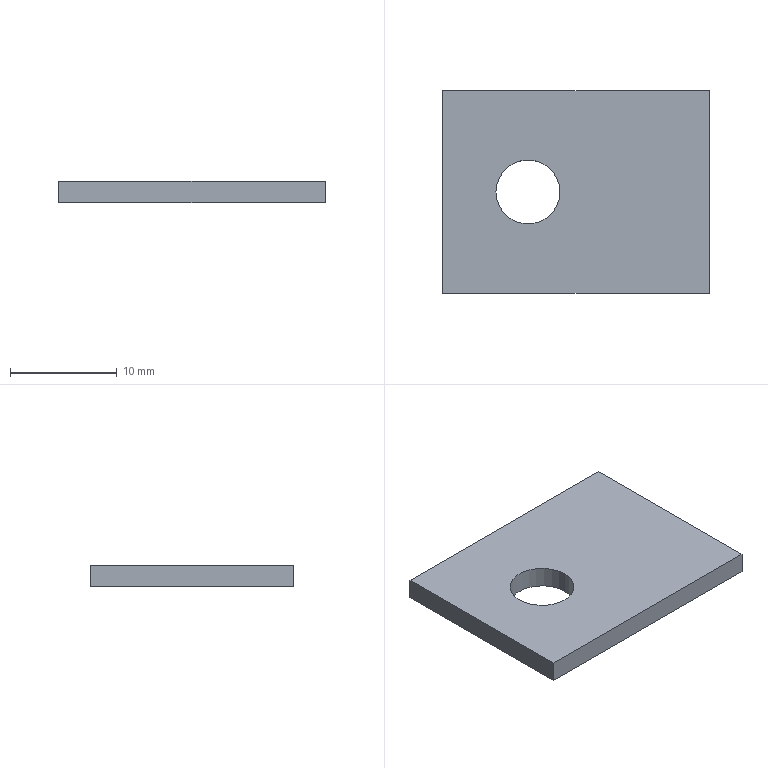Part | STEP file | Door Clip | 1 solid | 8 faces | box 25 x 19 x 2 mm | volume 893.451 mm3 | plane 6 | cylinder 2 | commonest cylinder face diameters 6 x2
STEP:
#1=CARTESIAN_POINT('',(-1429.216,-370.598,-2.));
#2=VERTEX_POINT('',#1);
#3=CARTESIAN_POINT('',(-1435.216,-370.598,-2.));
#4=VERTEX_POINT('',#3);
#5=CARTESIAN_POINT('',(-1432.216,-370.598,-2.));
#6=DIRECTION('',(0.,0.,-1.));
#7=DIRECTION('',(1.,0.,0.));
#8=AXIS2_PLACEMENT_3D('',#5,#6,#7);
#9=CIRCLE('',#8,3.);
#10=EDGE_CURVE('',#2,#4,#9,.T.);
#11=ORIENTED_EDGE('',*,*,#10,.T.);
#12=CARTESIAN_POINT('',(-1435.216,-370.598,0.));
#13=VERTEX_POINT('',#12);
#14=CARTESIAN_POINT('',(-1435.216,-370.598,-2.));
#15=DIRECTION('',(0.,0.,1.));
#16=VECTOR('',#15,1000.);
#17=LINE('',#14,#16);
#18=EDGE_CURVE('',#4,#13,#17,.T.);
#19=ORIENTED_EDGE('',*,*,#18,.T.);
#20=CARTESIAN_POINT('',(-1429.216,-370.598,0.));
#21=VERTEX_POINT('',#20);
#22=CARTESIAN_POINT('',(-1432.216,-370.598,0.));
#23=DIRECTION('',(0.,0.,-1.));
#24=DIRECTION('',(1.,0.,0.));
#25=AXIS2_PLACEMENT_3D('',#22,#23,#24);
#26=CIRCLE('',#25,3.);
#27=EDGE_CURVE('',#21,#13,#26,.T.);
#28=ORIENTED_EDGE('',*,*,#27,.F.);
#29=CARTESIAN_POINT('',(-1429.216,-370.598,-2.));
#30=DIRECTION('',(0.,0.,1.));
#31=VECTOR('',#30,1000.);
#32=LINE('',#29,#31);
#33=EDGE_CURVE('',#2,#21,#32,.T.);
#34=ORIENTED_EDGE('',*,*,#33,.F.);
#35=EDGE_LOOP('',(#11,#19,#28,#34));
#36=FACE_OUTER_BOUND('',#35,.T.);
#37=CARTESIAN_POINT('',(-1432.216,-370.598,-2.));
#38=DIRECTION('',(0.,0.,1.));
#39=DIRECTION('',(1.,0.,0.));
#40=AXIS2_PLACEMENT_3D('',#37,#38,#39);
#41=CYLINDRICAL_SURFACE('',#40,3.);
#42=ADVANCED_FACE('',(#36),#41,.F.);
#43=CARTESIAN_POINT('',(-1415.216,-361.098,-2.));
#44=VERTEX_POINT('',#43);
#45=CARTESIAN_POINT('',(-1440.216,-361.098,-2.));
#46=VERTEX_POINT('',#45);
#47=CARTESIAN_POINT('',(0.,-361.098,-2.));
#48=DIRECTION('',(-1.,0.,0.));
#49=VECTOR('',#48,1000.);
#50=LINE('',#47,#49);
#51=EDGE_CURVE('',#44,#46,#50,.T.);
#52=ORIENTED_EDGE('',*,*,#51,.F.);
#53=CARTESIAN_POINT('',(-1415.216,-380.098,-2.));
#54=VERTEX_POINT('',#53);
#55=CARTESIAN_POINT('',(-1415.216,0.,-2.));
#56=DIRECTION('',(0.,1.,0.));
#57=VECTOR('',#56,1000.);
#58=LINE('',#55,#57);
#59=EDGE_CURVE('',#54,#44,#58,.T.);
#60=ORIENTED_EDGE('',*,*,#59,.F.);
#61=CARTESIAN_POINT('',(-1440.216,-380.098,-2.));
#62=VERTEX_POINT('',#61);
#63=CARTESIAN_POINT('',(0.,-380.098,-2.));
#64=DIRECTION('',(1.,0.,0.));
#65=VECTOR('',#64,1000.);
#66=LINE('',#63,#65);
#67=EDGE_CURVE('',#62,#54,#66,.T.);
#68=ORIENTED_EDGE('',*,*,#67,.F.);
#69=CARTESIAN_POINT('',(-1440.216,0.,-2.));
#70=DIRECTION('',(0.,-1.,0.));
#71=VECTOR('',#70,1000.);
#72=LINE('',#69,#71);
#73=EDGE_CURVE('',#46,#62,#72,.T.);
#74=ORIENTED_EDGE('',*,*,#73,.F.);
#75=EDGE_LOOP('',(#52,#60,#68,#74));
#76=FACE_OUTER_BOUND('',#75,.T.);
#77=ORIENTED_EDGE('',*,*,#10,.F.);
#78=CARTESIAN_POINT('',(-1432.216,-370.598,-2.));
#79=DIRECTION('',(0.,0.,-1.));
#80=DIRECTION('',(1.,0.,0.));
#81=AXIS2_PLACEMENT_3D('',#78,#79,#80);
#82=CIRCLE('',#81,3.);
#83=EDGE_CURVE('',#4,#2,#82,.T.);
#84=ORIENTED_EDGE('',*,*,#83,.F.);
#85=EDGE_LOOP('',(#77,#84));
#86=FACE_BOUND('',#85,.T.);
#87=CARTESIAN_POINT('',(0.,0.,-2.));
#88=DIRECTION('',(0.,0.,1.));
#89=DIRECTION('',(1.,0.,0.));
#90=AXIS2_PLACEMENT_3D('',#87,#88,#89);
#91=PLANE('',#90);
#92=ADVANCED_FACE('',(#76,#86),#91,.F.);
#93=ORIENTED_EDGE('',*,*,#73,.T.);
#94=CARTESIAN_POINT('',(-1440.216,-380.098,0.));
#95=VERTEX_POINT('',#94);
#96=CARTESIAN_POINT('',(-1440.216,-380.098,-2.));
#97=DIRECTION('',(0.,0.,1.));
#98=VECTOR('',#97,1000.);
#99=LINE('',#96,#98);
#100=EDGE_CURVE('',#62,#95,#99,.T.);
#101=ORIENTED_EDGE('',*,*,#100,.T.);
#102=CARTESIAN_POINT('',(-1440.216,-361.098,0.));
#103=VERTEX_POINT('',#102);
#104=CARTESIAN_POINT('',(-1440.216,-361.098,0.));
#105=DIRECTION('',(0.,1.,0.));
#106=VECTOR('',#105,1000.);
#107=LINE('',#104,#106);
#108=EDGE_CURVE('',#95,#103,#107,.T.);
#109=ORIENTED_EDGE('',*,*,#108,.T.);
#110=CARTESIAN_POINT('',(-1440.216,-361.098,-2.));
#111=DIRECTION('',(0.,0.,-1.));
#112=VECTOR('',#111,1000.);
#113=LINE('',#110,#112);
#114=EDGE_CURVE('',#103,#46,#113,.T.);
#115=ORIENTED_EDGE('',*,*,#114,.T.);
#116=EDGE_LOOP('',(#93,#101,#109,#115));
#117=FACE_OUTER_BOUND('',#116,.T.);
#118=CARTESIAN_POINT('',(-1440.216,-361.098,-2.));
#119=DIRECTION('',(-1.,0.,0.));
#120=DIRECTION('',(0.,0.,1.));
#121=AXIS2_PLACEMENT_3D('',#118,#119,#120);
#122=PLANE('',#121);
#123=ADVANCED_FACE('',(#117),#122,.T.);
#124=ORIENTED_EDGE('',*,*,#51,.T.);
#125=ORIENTED_EDGE('',*,*,#114,.F.);
#126=CARTESIAN_POINT('',(-1415.216,-361.098,0.));
#127=VERTEX_POINT('',#126);
#128=CARTESIAN_POINT('',(-1440.216,-361.098,0.));
#129=DIRECTION('',(1.,0.,0.));
#130=VECTOR('',#129,1000.);
#131=LINE('',#128,#130);
#132=EDGE_CURVE('',#103,#127,#131,.T.);
#133=ORIENTED_EDGE('',*,*,#132,.T.);
#134=CARTESIAN_POINT('',(-1415.216,-361.098,-2.));
#135=DIRECTION('',(0.,0.,-1.));
#136=VECTOR('',#135,1000.);
#137=LINE('',#134,#136);
#138=EDGE_CURVE('',#127,#44,#137,.T.);
#139=ORIENTED_EDGE('',*,*,#138,.T.);
#140=EDGE_LOOP('',(#124,#125,#133,#139));
#141=FACE_OUTER_BOUND('',#140,.T.);
#142=CARTESIAN_POINT('',(-1440.216,-361.098,-2.));
#143=DIRECTION('',(0.,1.,0.));
#144=DIRECTION('',(0.,0.,1.));
#145=AXIS2_PLACEMENT_3D('',#142,#143,#144);
#146=PLANE('',#145);
#147=ADVANCED_FACE('',(#141),#146,.T.);
#148=ORIENTED_EDGE('',*,*,#59,.T.);
#149=ORIENTED_EDGE('',*,*,#138,.F.);
#150=CARTESIAN_POINT('',(-1415.216,-380.098,0.));
#151=VERTEX_POINT('',#150);
#152=CARTESIAN_POINT('',(-1415.216,-361.098,0.));
#153=DIRECTION('',(0.,-1.,0.));
#154=VECTOR('',#153,1000.);
#155=LINE('',#152,#154);
#156=EDGE_CURVE('',#127,#151,#155,.T.);
#157=ORIENTED_EDGE('',*,*,#156,.T.);
#158=CARTESIAN_POINT('',(-1415.216,-380.098,-2.));
#159=DIRECTION('',(0.,0.,-1.));
#160=VECTOR('',#159,1000.);
#161=LINE('',#158,#160);
#162=EDGE_CURVE('',#151,#54,#161,.T.);
#163=ORIENTED_EDGE('',*,*,#162,.T.);
#164=EDGE_LOOP('',(#148,#149,#157,#163));
#165=FACE_OUTER_BOUND('',#164,.T.);
#166=CARTESIAN_POINT('',(-1415.216,-361.098,-2.));
#167=DIRECTION('',(1.,0.,0.));
#168=DIRECTION('',(0.,0.,-1.));
#169=AXIS2_PLACEMENT_3D('',#166,#167,#168);
#170=PLANE('',#169);
#171=ADVANCED_FACE('',(#165),#170,.T.);
#172=ORIENTED_EDGE('',*,*,#67,.T.);
#173=ORIENTED_EDGE('',*,*,#162,.F.);
#174=CARTESIAN_POINT('',(-1440.216,-380.098,0.));
#175=DIRECTION('',(-1.,0.,0.));
#176=VECTOR('',#175,1000.);
#177=LINE('',#174,#176);
#178=EDGE_CURVE('',#151,#95,#177,.T.);
#179=ORIENTED_EDGE('',*,*,#178,.T.);
#180=ORIENTED_EDGE('',*,*,#100,.F.);
#181=EDGE_LOOP('',(#172,#173,#179,#180));
#182=FACE_OUTER_BOUND('',#181,.T.);
#183=CARTESIAN_POINT('',(-1440.216,-380.098,-2.));
#184=DIRECTION('',(0.,-1.,0.));
#185=DIRECTION('',(0.,0.,-1.));
#186=AXIS2_PLACEMENT_3D('',#183,#184,#185);
#187=PLANE('',#186);
#188=ADVANCED_FACE('',(#182),#187,.T.);
#189=ORIENTED_EDGE('',*,*,#18,.F.);
#190=ORIENTED_EDGE('',*,*,#83,.T.);
#191=ORIENTED_EDGE('',*,*,#33,.T.);
#192=CARTESIAN_POINT('',(-1432.216,-370.598,0.));
#193=DIRECTION('',(0.,0.,-1.));
#194=DIRECTION('',(1.,0.,0.));
#195=AXIS2_PLACEMENT_3D('',#192,#193,#194);
#196=CIRCLE('',#195,3.);
#197=EDGE_CURVE('',#13,#21,#196,.T.);
#198=ORIENTED_EDGE('',*,*,#197,.F.);
#199=EDGE_LOOP('',(#189,#190,#191,#198));
#200=FACE_OUTER_BOUND('',#199,.T.);
#201=CARTESIAN_POINT('',(-1432.216,-370.598,-2.));
#202=DIRECTION('',(0.,0.,1.));
#203=DIRECTION('',(1.,0.,0.));
#204=AXIS2_PLACEMENT_3D('',#201,#202,#203);
#205=CYLINDRICAL_SURFACE('',#204,3.);
#206=ADVANCED_FACE('',(#200),#205,.F.);
#207=ORIENTED_EDGE('',*,*,#156,.F.);
#208=ORIENTED_EDGE('',*,*,#132,.F.);
#209=ORIENTED_EDGE('',*,*,#108,.F.);
#210=ORIENTED_EDGE('',*,*,#178,.F.);
#211=EDGE_LOOP('',(#207,#208,#209,#210));
#212=FACE_OUTER_BOUND('',#211,.T.);
#213=ORIENTED_EDGE('',*,*,#27,.T.);
#214=ORIENTED_EDGE('',*,*,#197,.T.);
#215=EDGE_LOOP('',(#213,#214));
#216=FACE_BOUND('',#215,.T.);
#217=CARTESIAN_POINT('',(0.,0.,0.));
#218=DIRECTION('',(0.,0.,1.));
#219=DIRECTION('',(1.,0.,0.));
#220=AXIS2_PLACEMENT_3D('',#217,#218,#219);
#221=PLANE('',#220);
#222=ADVANCED_FACE('',(#212,#216),#221,.T.);
#223=CLOSED_SHELL('',(#42,#92,#123,#147,#171,#188,#206,#222));
#224=MANIFOLD_SOLID_BREP('',#223);
#225=CARTESIAN_POINT('',(0.,0.,0.));
#226=DIRECTION('',(0.,0.,1.));
#227=DIRECTION('',(1.,0.,0.));
#228=AXIS2_PLACEMENT_3D('',#225,#226,#227);
#229=(LENGTH_UNIT()NAMED_UNIT(*)SI_UNIT(.MILLI.,.METRE.));
#230=UNCERTAINTY_MEASURE_WITH_UNIT(LENGTH_MEASURE(0.00001),#229,'','');
#231=(NAMED_UNIT(*)PLANE_ANGLE_UNIT()SI_UNIT($,.RADIAN.));
#232=(NAMED_UNIT(*)SI_UNIT($,.STERADIAN.)SOLID_ANGLE_UNIT());
#233=(GEOMETRIC_REPRESENTATION_CONTEXT(3)GLOBAL_UNCERTAINTY_ASSIGNED_CONTEXT((#230))GLOBAL_UNIT_ASSIGNED_CONTEXT((#229,#231,#232))REPRESENTATION_CONTEXT('',''));
#234=ADVANCED_BREP_SHAPE_REPRESENTATION('',(#224,#228),#233);